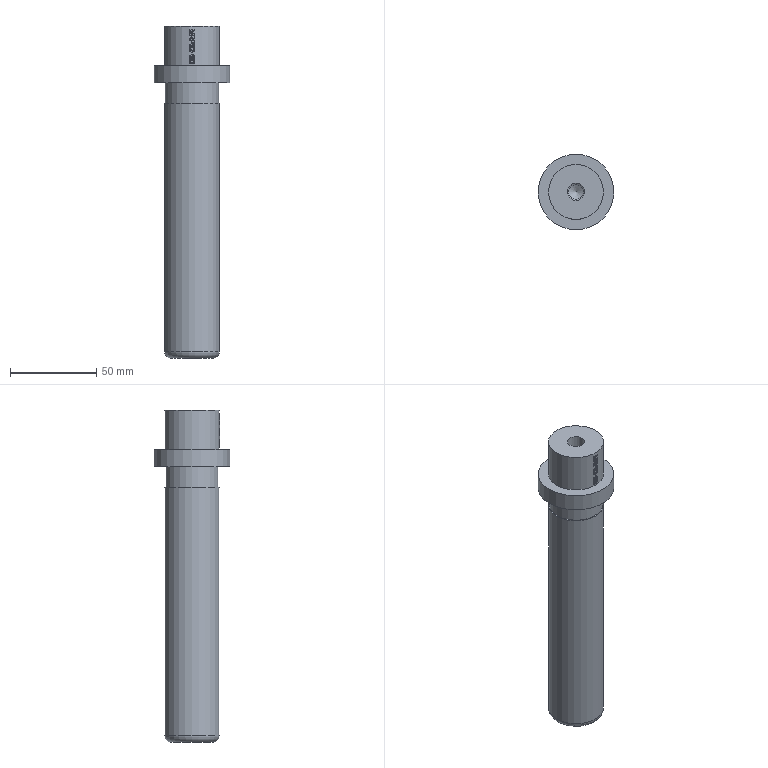Part | NX | features 18 2 | 1 solid | 134 faces | box 44 x 44 x 193 mm | volume 159798 mm3 | plane 73 | cylinder 58 | cone 2 | torus 1 | commonest cylinder face diameters 31.8 x9 32 x6 1.807 x2 1.017 x1 1.059 x1 1.062 x1